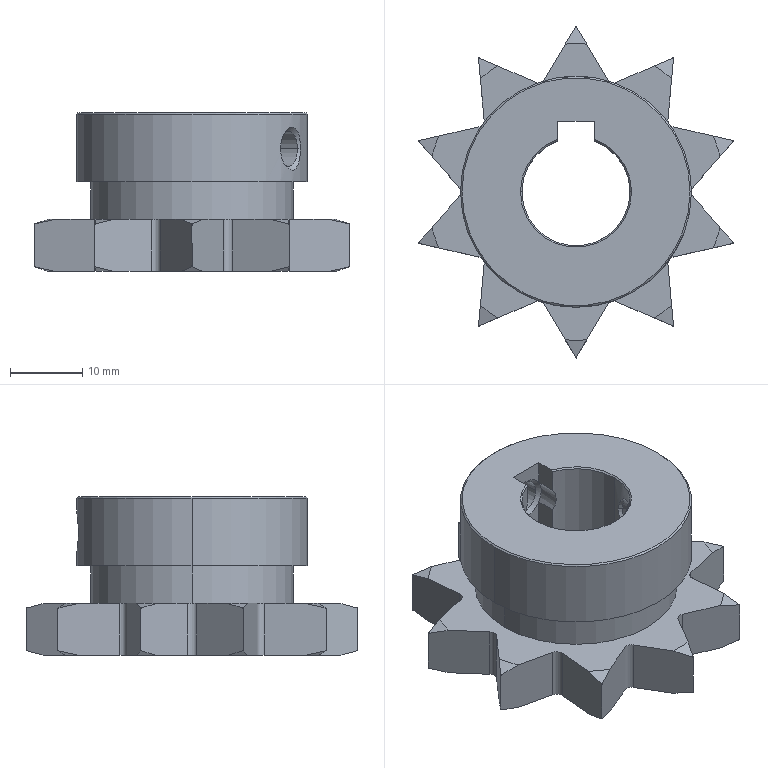Part | NX | features BREP 1 | 1 solid | 116 faces | box 43.749 x 46 x 22 mm | volume 14481 mm3 | cone 36 | cylinder 30 | plane 30 | torus 20 | commonest cylinder face diameters 2 x13 6 x6 4.917 x4 15 x3 28 x2 32 x2